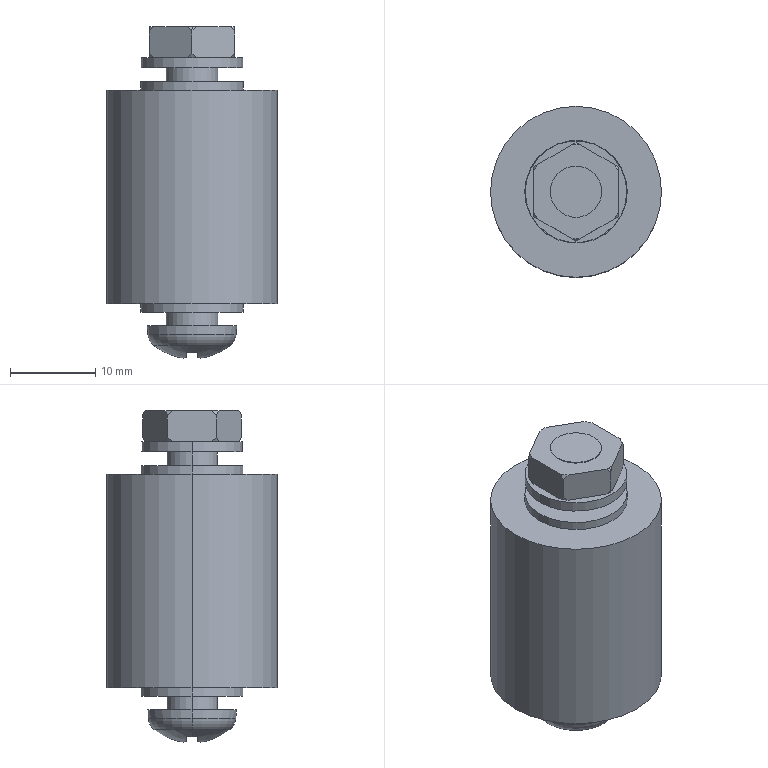Part | STEP file | Mirror ROLLER-1_0829_041_CRONWB29 | 1 solid | 66 faces | box 20 x 20 x 38.858 mm | volume 8836 mm3 | plane 28 | cylinder 18 | cone 16 | sphere 2 | torus 2 | commonest cylinder face diameters 6 x6 2 x4 12 x4 11.9 x2 20 x2